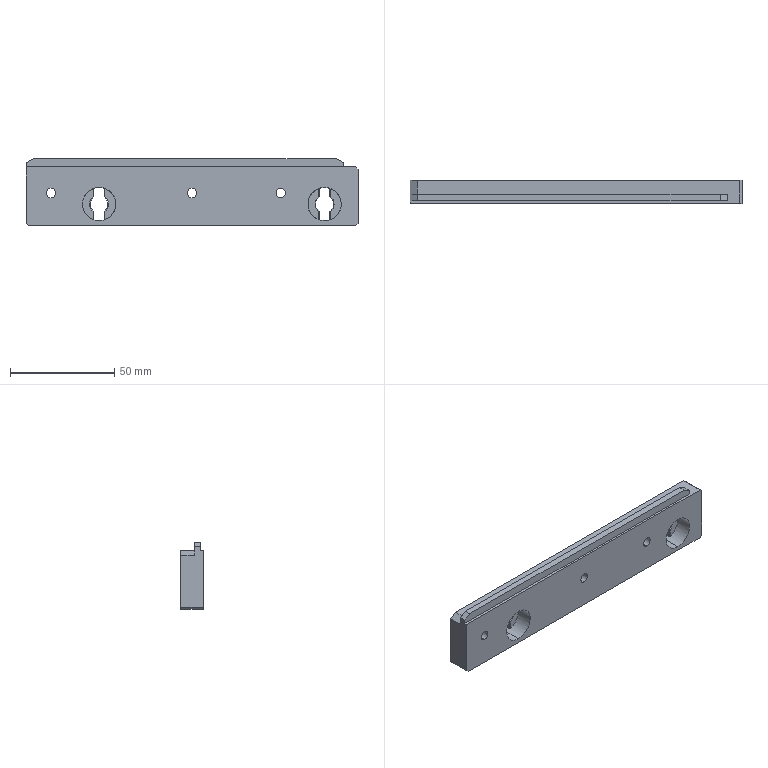Part | STEP file | FBDS-CS-007 | 1 solid | 85 faces | box 159 x 11 x 32 mm | volume 45788 mm3 | plane 47 | cylinder 22 | cone 16 | commonest cylinder face diameters 4.5 x6 8 x6 8.5 x4 16 x4 3.3 x2